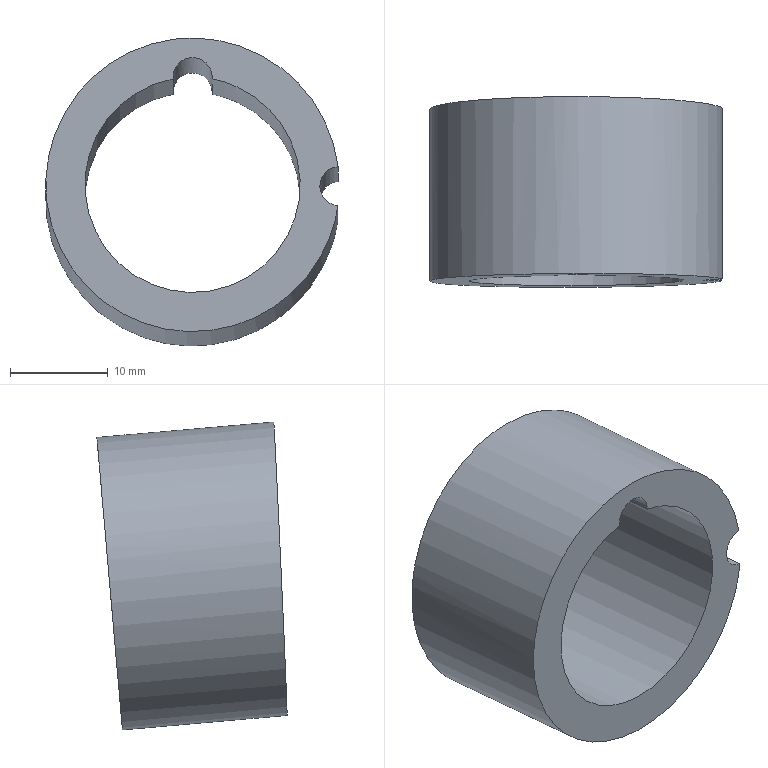Part | NX | features solid 2 | 1 solid | 6 faces | box 29.872 x 19.436 x 31.465 mm | volume 5378 mm3 | spline 2 | plane 2 | cylinder 2 | commonest cylinder face diameters 4 x2